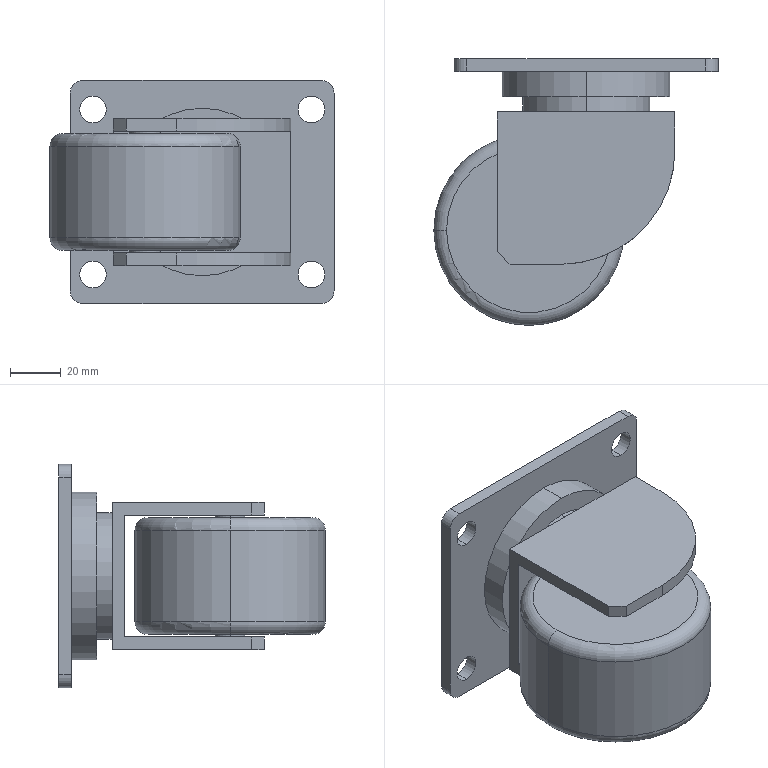Part | STEP file | 3 inch heavy-duty caster 7223-222B | 1 solid | 70 faces | box 112 x 105 x 88 mm | volume 158459 mm3 | cylinder 34 | plane 28 | torus 8 | commonest cylinder face diameters 10.5 x8 5.6 x4 10 x4 12 x4 43.6 x2 50 x2